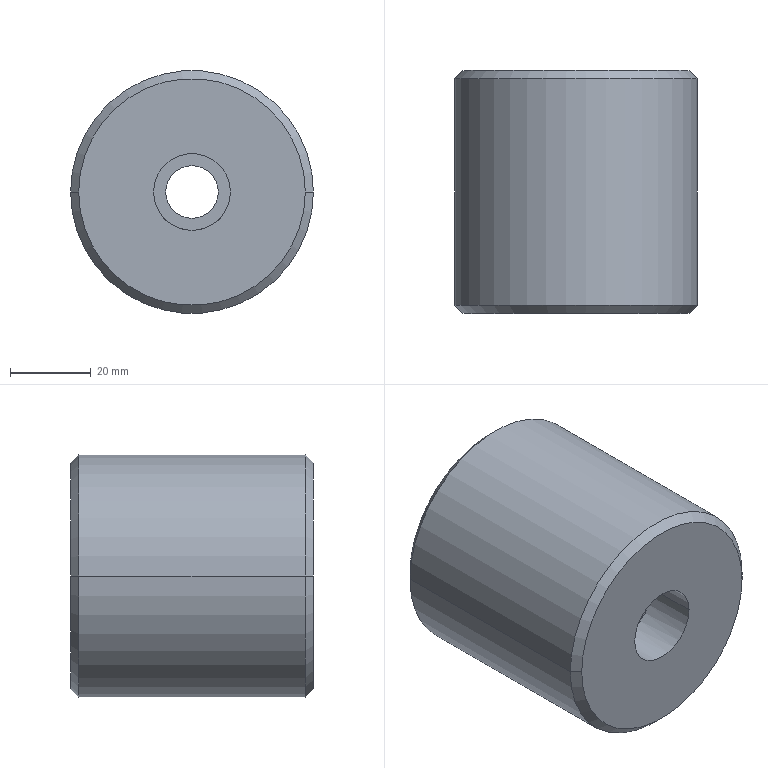Part | Creo | 1 solid | 13 faces | box 60 x 60 x 60 mm | volume 158984 mm3 | cylinder 6 | cone 4 | plane 3 | commonest cylinder face diameters 13 x2 19 x2 60 x2
STEP:
#1=CARTESIAN_POINT('',(278.,-435.005,80.));
#2=VERTEX_POINT('',#1);
#3=CARTESIAN_POINT('',(222.,-435.005,80.));
#4=VERTEX_POINT('',#3);
#5=CARTESIAN_POINT('',(250.,-435.005,80.));
#6=DIRECTION('',(0.,-1.,0.));
#7=DIRECTION('',(1.,0.,0.));
#8=AXIS2_PLACEMENT_3D('',#5,#6,#7);
#9=CIRCLE('',#8,28.);
#10=EDGE_CURVE('',#2,#4,#9,.T.);
#11=ORIENTED_EDGE('',*,*,#10,.F.);
#12=CARTESIAN_POINT('',(250.,-435.005,80.));
#13=DIRECTION('',(0.,-1.,0.));
#14=DIRECTION('',(-1.,0.,0.));
#15=AXIS2_PLACEMENT_3D('',#12,#13,#14);
#16=CIRCLE('',#15,28.);
#17=EDGE_CURVE('',#4,#2,#16,.T.);
#18=ORIENTED_EDGE('',*,*,#17,.F.);
#19=EDGE_LOOP('',(#11,#18));
#20=FACE_OUTER_BOUND('',#19,.F.);
#21=CARTESIAN_POINT('',(250.,-435.005,70.5));
#22=VERTEX_POINT('',#21);
#23=CARTESIAN_POINT('',(240.5,-435.005,80.));
#24=VERTEX_POINT('',#23);
#25=CARTESIAN_POINT('',(250.,-435.005,80.));
#26=DIRECTION('',(0.,1.,0.));
#27=DIRECTION('',(0.,0.,-1.));
#28=AXIS2_PLACEMENT_3D('',#25,#26,#27);
#29=CIRCLE('',#28,9.5);
#30=EDGE_CURVE('',#22,#24,#29,.T.);
#31=ORIENTED_EDGE('',*,*,#30,.F.);
#32=CARTESIAN_POINT('',(259.5,-435.005,80.));
#33=VERTEX_POINT('',#32);
#34=CARTESIAN_POINT('',(250.,-435.005,80.));
#35=DIRECTION('',(0.,1.,0.));
#36=DIRECTION('',(1.,0.,0.));
#37=AXIS2_PLACEMENT_3D('',#34,#35,#36);
#38=CIRCLE('',#37,9.5);
#39=EDGE_CURVE('',#33,#22,#38,.T.);
#40=ORIENTED_EDGE('',*,*,#39,.F.);
#41=CARTESIAN_POINT('',(250.,-435.005,80.));
#42=DIRECTION('',(0.,1.,0.));
#43=DIRECTION('',(-1.,0.,0.));
#44=AXIS2_PLACEMENT_3D('',#41,#42,#43);
#45=CIRCLE('',#44,9.5);
#46=EDGE_CURVE('',#24,#33,#45,.T.);
#47=ORIENTED_EDGE('',*,*,#46,.F.);
#48=EDGE_LOOP('',(#31,#40,#47));
#49=FACE_BOUND('',#48,.F.);
#50=CARTESIAN_POINT('',(10.,-435.005,-351.));
#51=DIRECTION('',(0.,-1.,0.));
#52=DIRECTION('',(1.,0.,0.));
#53=AXIS2_PLACEMENT_3D('',#50,#51,#52);
#54=PLANE('',#53);
#55=ADVANCED_FACE('',(#20,#49),#54,.T.);
#56=ORIENTED_EDGE('',*,*,#39,.T.);
#57=ORIENTED_EDGE('',*,*,#30,.T.);
#58=CARTESIAN_POINT('',(240.5,-422.005,80.));
#59=VERTEX_POINT('',#58);
#60=CARTESIAN_POINT('',(240.5,-435.005,80.));
#61=DIRECTION('',(0.,1.,0.));
#62=VECTOR('',#61,13.);
#63=LINE('',#60,#62);
#64=EDGE_CURVE('',#24,#59,#63,.T.);
#65=ORIENTED_EDGE('',*,*,#64,.T.);
#66=CARTESIAN_POINT('',(259.5,-422.005,80.));
#67=VERTEX_POINT('',#66);
#68=CARTESIAN_POINT('',(250.,-422.005,80.));
#69=DIRECTION('',(0.,-1.,0.));
#70=DIRECTION('',(-1.,0.,0.));
#71=AXIS2_PLACEMENT_3D('',#68,#69,#70);
#72=CIRCLE('',#71,9.5);
#73=EDGE_CURVE('',#59,#67,#72,.T.);
#74=ORIENTED_EDGE('',*,*,#73,.T.);
#75=CARTESIAN_POINT('',(259.5,-435.005,80.));
#76=DIRECTION('',(0.,1.,0.));
#77=VECTOR('',#76,13.);
#78=LINE('',#75,#77);
#79=EDGE_CURVE('',#33,#67,#78,.T.);
#80=ORIENTED_EDGE('',*,*,#79,.F.);
#81=EDGE_LOOP('',(#56,#57,#65,#74,#80));
#82=FACE_OUTER_BOUND('',#81,.F.);
#83=CARTESIAN_POINT('',(250.,-447.005,80.));
#84=DIRECTION('',(0.,1.,0.));
#85=DIRECTION('',(1.,0.,0.));
#86=AXIS2_PLACEMENT_3D('',#83,#84,#85);
#87=CYLINDRICAL_SURFACE('',#86,9.5);
#88=ADVANCED_FACE('',(#82),#87,.F.);
#89=ORIENTED_EDGE('',*,*,#46,.T.);
#90=ORIENTED_EDGE('',*,*,#79,.T.);
#91=CARTESIAN_POINT('',(250.,-422.005,80.));
#92=DIRECTION('',(0.,-1.,0.));
#93=DIRECTION('',(1.,0.,0.));
#94=AXIS2_PLACEMENT_3D('',#91,#92,#93);
#95=CIRCLE('',#94,9.5);
#96=EDGE_CURVE('',#67,#59,#95,.T.);
#97=ORIENTED_EDGE('',*,*,#96,.T.);
#98=ORIENTED_EDGE('',*,*,#64,.F.);
#99=EDGE_LOOP('',(#89,#90,#97,#98));
#100=FACE_OUTER_BOUND('',#99,.F.);
#101=CARTESIAN_POINT('',(250.,-447.005,80.));
#102=DIRECTION('',(0.,1.,0.));
#103=DIRECTION('',(1.,0.,0.));
#104=AXIS2_PLACEMENT_3D('',#101,#102,#103);
#105=CYLINDRICAL_SURFACE('',#104,9.5);
#106=ADVANCED_FACE('',(#100),#105,.F.);
#107=ORIENTED_EDGE('',*,*,#96,.F.);
#108=ORIENTED_EDGE('',*,*,#73,.F.);
#109=EDGE_LOOP('',(#107,#108));
#110=FACE_OUTER_BOUND('',#109,.F.);
#111=CARTESIAN_POINT('',(250.,-422.005,86.5));
#112=VERTEX_POINT('',#111);
#113=CARTESIAN_POINT('',(256.5,-422.005,80.));
#114=VERTEX_POINT('',#113);
#115=CARTESIAN_POINT('',(250.,-422.005,80.));
#116=DIRECTION('',(0.,1.,0.));
#117=DIRECTION('',(0.,0.,1.));
#118=AXIS2_PLACEMENT_3D('',#115,#116,#117);
#119=CIRCLE('',#118,6.5);
#120=EDGE_CURVE('',#112,#114,#119,.T.);
#121=ORIENTED_EDGE('',*,*,#120,.F.);
#122=CARTESIAN_POINT('',(243.5,-422.005,80.));
#123=VERTEX_POINT('',#122);
#124=CARTESIAN_POINT('',(250.,-422.005,80.));
#125=DIRECTION('',(0.,1.,0.));
#126=DIRECTION('',(-1.,0.,0.));
#127=AXIS2_PLACEMENT_3D('',#124,#125,#126);
#128=CIRCLE('',#127,6.5);
#129=EDGE_CURVE('',#123,#112,#128,.T.);
#130=ORIENTED_EDGE('',*,*,#129,.F.);
#131=CARTESIAN_POINT('',(250.,-422.005,73.5));
#132=VERTEX_POINT('',#131);
#133=CARTESIAN_POINT('',(250.,-422.005,80.));
#134=DIRECTION('',(0.,1.,0.));
#135=DIRECTION('',(0.,0.,-1.));
#136=AXIS2_PLACEMENT_3D('',#133,#134,#135);
#137=CIRCLE('',#136,6.5);
#138=EDGE_CURVE('',#132,#123,#137,.T.);
#139=ORIENTED_EDGE('',*,*,#138,.F.);
#140=CARTESIAN_POINT('',(250.,-422.005,80.));
#141=DIRECTION('',(0.,1.,0.));
#142=DIRECTION('',(1.,0.,0.));
#143=AXIS2_PLACEMENT_3D('',#140,#141,#142);
#144=CIRCLE('',#143,6.5);
#145=EDGE_CURVE('',#114,#132,#144,.T.);
#146=ORIENTED_EDGE('',*,*,#145,.F.);
#147=EDGE_LOOP('',(#121,#130,#139,#146));
#148=FACE_BOUND('',#147,.F.);
#149=CARTESIAN_POINT('',(250.,-422.005,80.));
#150=DIRECTION('',(0.,1.,0.));
#151=DIRECTION('',(0.,0.,1.));
#152=AXIS2_PLACEMENT_3D('',#149,#150,#151);
#153=PLANE('',#152);
#154=ADVANCED_FACE('',(#110,#148),#153,.F.);
#155=ORIENTED_EDGE('',*,*,#129,.T.);
#156=ORIENTED_EDGE('',*,*,#120,.T.);
#157=CARTESIAN_POINT('',(256.5,-375.005,80.));
#158=VERTEX_POINT('',#157);
#159=CARTESIAN_POINT('',(256.5,-422.005,80.));
#160=DIRECTION('',(0.,1.,0.));
#161=VECTOR('',#160,47.);
#162=LINE('',#159,#161);
#163=EDGE_CURVE('',#114,#158,#162,.T.);
#164=ORIENTED_EDGE('',*,*,#163,.T.);
#165=CARTESIAN_POINT('',(243.5,-375.005,80.));
#166=VERTEX_POINT('',#165);
#167=CARTESIAN_POINT('',(250.,-375.005,80.));
#168=DIRECTION('',(0.,-1.,0.));
#169=DIRECTION('',(1.,0.,0.));
#170=AXIS2_PLACEMENT_3D('',#167,#168,#169);
#171=CIRCLE('',#170,6.5);
#172=EDGE_CURVE('',#158,#166,#171,.T.);
#173=ORIENTED_EDGE('',*,*,#172,.T.);
#174=CARTESIAN_POINT('',(243.5,-422.005,80.));
#175=DIRECTION('',(0.,1.,0.));
#176=VECTOR('',#175,47.);
#177=LINE('',#174,#176);
#178=EDGE_CURVE('',#123,#166,#177,.T.);
#179=ORIENTED_EDGE('',*,*,#178,.F.);
#180=EDGE_LOOP('',(#155,#156,#164,#173,#179));
#181=FACE_OUTER_BOUND('',#180,.F.);
#182=CARTESIAN_POINT('',(250.,-447.005,80.));
#183=DIRECTION('',(0.,1.,0.));
#184=DIRECTION('',(1.,0.,0.));
#185=AXIS2_PLACEMENT_3D('',#182,#183,#184);
#186=CYLINDRICAL_SURFACE('',#185,6.5);
#187=ADVANCED_FACE('',(#181),#186,.F.);
#188=ORIENTED_EDGE('',*,*,#138,.T.);
#189=ORIENTED_EDGE('',*,*,#178,.T.);
#190=CARTESIAN_POINT('',(250.,-375.005,80.));
#191=DIRECTION('',(0.,-1.,0.));
#192=DIRECTION('',(-1.,0.,0.));
#193=AXIS2_PLACEMENT_3D('',#190,#191,#192);
#194=CIRCLE('',#193,6.5);
#195=EDGE_CURVE('',#166,#158,#194,.T.);
#196=ORIENTED_EDGE('',*,*,#195,.T.);
#197=ORIENTED_EDGE('',*,*,#163,.F.);
#198=ORIENTED_EDGE('',*,*,#145,.T.);
#199=EDGE_LOOP('',(#188,#189,#196,#197,#198));
#200=FACE_OUTER_BOUND('',#199,.F.);
#201=CARTESIAN_POINT('',(250.,-447.005,80.));
#202=DIRECTION('',(0.,1.,0.));
#203=DIRECTION('',(1.,0.,0.));
#204=AXIS2_PLACEMENT_3D('',#201,#202,#203);
#205=CYLINDRICAL_SURFACE('',#204,6.5);
#206=ADVANCED_FACE('',(#200),#205,.F.);
#207=CARTESIAN_POINT('',(222.,-375.005,80.));
#208=VERTEX_POINT('',#207);
#209=CARTESIAN_POINT('',(278.,-375.005,80.));
#210=VERTEX_POINT('',#209);
#211=CARTESIAN_POINT('',(250.,-375.005,80.));
#212=DIRECTION('',(0.,1.,0.));
#213=DIRECTION('',(-1.,0.,0.));
#214=AXIS2_PLACEMENT_3D('',#211,#212,#213);
#215=CIRCLE('',#214,28.);
#216=EDGE_CURVE('',#208,#210,#215,.T.);
#217=ORIENTED_EDGE('',*,*,#216,.F.);
#218=CARTESIAN_POINT('',(250.,-375.005,80.));
#219=DIRECTION('',(0.,1.,0.));
#220=DIRECTION('',(1.,0.,0.));
#221=AXIS2_PLACEMENT_3D('',#218,#219,#220);
#222=CIRCLE('',#221,28.);
#223=EDGE_CURVE('',#210,#208,#222,.T.);
#224=ORIENTED_EDGE('',*,*,#223,.F.);
#225=EDGE_LOOP('',(#217,#224));
#226=FACE_OUTER_BOUND('',#225,.F.);
#227=ORIENTED_EDGE('',*,*,#172,.F.);
#228=ORIENTED_EDGE('',*,*,#195,.F.);
#229=EDGE_LOOP('',(#227,#228));
#230=FACE_BOUND('',#229,.F.);
#231=CARTESIAN_POINT('',(10.,-375.005,-351.));
#232=DIRECTION('',(0.,-1.,0.));
#233=DIRECTION('',(1.,0.,0.));
#234=AXIS2_PLACEMENT_3D('',#231,#232,#233);
#235=PLANE('',#234);
#236=ADVANCED_FACE('',(#226,#230),#235,.F.);
#237=CARTESIAN_POINT('',(220.,-377.005,80.));
#238=VERTEX_POINT('',#237);
#239=CARTESIAN_POINT('',(280.,-377.005,80.));
#240=VERTEX_POINT('',#239);
#241=CARTESIAN_POINT('',(250.,-377.005,80.));
#242=DIRECTION('',(0.,1.,0.));
#243=DIRECTION('',(-1.,0.,0.));
#244=AXIS2_PLACEMENT_3D('',#241,#242,#243);
#245=CIRCLE('',#244,30.);
#246=EDGE_CURVE('',#238,#240,#245,.T.);
#247=ORIENTED_EDGE('',*,*,#246,.F.);
#248=CARTESIAN_POINT('',(222.,-375.005,80.));
#249=DIRECTION('',(-0.7071,-0.7071,0.));
#250=VECTOR('',#249,2.828);
#251=LINE('',#248,#250);
#252=EDGE_CURVE('',#208,#238,#251,.T.);
#253=ORIENTED_EDGE('',*,*,#252,.F.);
#254=ORIENTED_EDGE('',*,*,#216,.T.);
#255=CARTESIAN_POINT('',(278.,-375.005,80.));
#256=DIRECTION('',(0.7071,-0.7071,0.));
#257=VECTOR('',#256,2.828);
#258=LINE('',#255,#257);
#259=EDGE_CURVE('',#210,#240,#258,.T.);
#260=ORIENTED_EDGE('',*,*,#259,.T.);
#261=EDGE_LOOP('',(#247,#253,#254,#260));
#262=FACE_OUTER_BOUND('',#261,.F.);
#263=CARTESIAN_POINT('',(250.,-376.005,80.));
#264=DIRECTION('',(0.,-1.,0.));
#265=DIRECTION('',(-1.,0.,0.));
#266=AXIS2_PLACEMENT_3D('',#263,#264,#265);
#267=CONICAL_SURFACE('',#266,29.,45.);
#268=ADVANCED_FACE('',(#262),#267,.T.);
#269=ORIENTED_EDGE('',*,*,#246,.T.);
#270=CARTESIAN_POINT('',(280.,-433.005,80.));
#271=VERTEX_POINT('',#270);
#272=CARTESIAN_POINT('',(280.,-377.005,80.));
#273=DIRECTION('',(0.,-1.,0.));
#274=VECTOR('',#273,56.);
#275=LINE('',#272,#274);
#276=EDGE_CURVE('',#240,#271,#275,.T.);
#277=ORIENTED_EDGE('',*,*,#276,.T.);
#278=CARTESIAN_POINT('',(220.,-433.005,80.));
#279=VERTEX_POINT('',#278);
#280=CARTESIAN_POINT('',(250.,-433.005,80.));
#281=DIRECTION('',(0.,-1.,0.));
#282=DIRECTION('',(1.,0.,0.));
#283=AXIS2_PLACEMENT_3D('',#280,#281,#282);
#284=CIRCLE('',#283,30.);
#285=EDGE_CURVE('',#271,#279,#284,.T.);
#286=ORIENTED_EDGE('',*,*,#285,.T.);
#287=CARTESIAN_POINT('',(220.,-377.005,80.));
#288=DIRECTION('',(0.,-1.,0.));
#289=VECTOR('',#288,56.);
#290=LINE('',#287,#289);
#291=EDGE_CURVE('',#238,#279,#290,.T.);
#292=ORIENTED_EDGE('',*,*,#291,.F.);
#293=EDGE_LOOP('',(#269,#277,#286,#292));
#294=FACE_OUTER_BOUND('',#293,.F.);
#295=CARTESIAN_POINT('',(250.,-375.005,80.));
#296=DIRECTION('',(0.,-1.,0.));
#297=DIRECTION('',(1.,0.,0.));
#298=AXIS2_PLACEMENT_3D('',#295,#296,#297);
#299=CYLINDRICAL_SURFACE('',#298,30.);
#300=ADVANCED_FACE('',(#294),#299,.T.);
#301=CARTESIAN_POINT('',(250.,-377.005,80.));
#302=DIRECTION('',(0.,1.,0.));
#303=DIRECTION('',(1.,0.,0.));
#304=AXIS2_PLACEMENT_3D('',#301,#302,#303);
#305=CIRCLE('',#304,30.);
#306=EDGE_CURVE('',#240,#238,#305,.T.);
#307=ORIENTED_EDGE('',*,*,#306,.T.);
#308=ORIENTED_EDGE('',*,*,#291,.T.);
#309=CARTESIAN_POINT('',(250.,-433.005,80.));
#310=DIRECTION('',(0.,-1.,0.));
#311=DIRECTION('',(-1.,0.,0.));
#312=AXIS2_PLACEMENT_3D('',#309,#310,#311);
#313=CIRCLE('',#312,30.);
#314=EDGE_CURVE('',#279,#271,#313,.T.);
#315=ORIENTED_EDGE('',*,*,#314,.T.);
#316=ORIENTED_EDGE('',*,*,#276,.F.);
#317=EDGE_LOOP('',(#307,#308,#315,#316));
#318=FACE_OUTER_BOUND('',#317,.F.);
#319=CARTESIAN_POINT('',(250.,-375.005,80.));
#320=DIRECTION('',(0.,-1.,0.));
#321=DIRECTION('',(1.,0.,0.));
#322=AXIS2_PLACEMENT_3D('',#319,#320,#321);
#323=CYLINDRICAL_SURFACE('',#322,30.);
#324=ADVANCED_FACE('',(#318),#323,.T.);
#325=ORIENTED_EDGE('',*,*,#306,.F.);
#326=ORIENTED_EDGE('',*,*,#259,.F.);
#327=ORIENTED_EDGE('',*,*,#223,.T.);
#328=ORIENTED_EDGE('',*,*,#252,.T.);
#329=EDGE_LOOP('',(#325,#326,#327,#328));
#330=FACE_OUTER_BOUND('',#329,.F.);
#331=CARTESIAN_POINT('',(250.,-376.005,80.));
#332=DIRECTION('',(0.,-1.,0.));
#333=DIRECTION('',(-1.,0.,0.));
#334=AXIS2_PLACEMENT_3D('',#331,#332,#333);
#335=CONICAL_SURFACE('',#334,29.,45.);
#336=ADVANCED_FACE('',(#330),#335,.T.);
#337=ORIENTED_EDGE('',*,*,#17,.T.);
#338=CARTESIAN_POINT('',(278.,-435.005,80.));
#339=DIRECTION('',(0.7071,0.7071,0.));
#340=VECTOR('',#339,2.828);
#341=LINE('',#338,#340);
#342=EDGE_CURVE('',#2,#271,#341,.T.);
#343=ORIENTED_EDGE('',*,*,#342,.T.);
#344=ORIENTED_EDGE('',*,*,#314,.F.);
#345=CARTESIAN_POINT('',(222.,-435.005,80.));
#346=DIRECTION('',(-0.7071,0.7071,0.));
#347=VECTOR('',#346,2.828);
#348=LINE('',#345,#347);
#349=EDGE_CURVE('',#4,#279,#348,.T.);
#350=ORIENTED_EDGE('',*,*,#349,.F.);
#351=EDGE_LOOP('',(#337,#343,#344,#350));
#352=FACE_OUTER_BOUND('',#351,.F.);
#353=CARTESIAN_POINT('',(250.,-434.005,80.));
#354=DIRECTION('',(0.,1.,0.));
#355=DIRECTION('',(-1.,0.,0.));
#356=AXIS2_PLACEMENT_3D('',#353,#354,#355);
#357=CONICAL_SURFACE('',#356,29.,45.);
#358=ADVANCED_FACE('',(#352),#357,.T.);
#359=ORIENTED_EDGE('',*,*,#10,.T.);
#360=ORIENTED_EDGE('',*,*,#349,.T.);
#361=ORIENTED_EDGE('',*,*,#285,.F.);
#362=ORIENTED_EDGE('',*,*,#342,.F.);
#363=EDGE_LOOP('',(#359,#360,#361,#362));
#364=FACE_OUTER_BOUND('',#363,.F.);
#365=CARTESIAN_POINT('',(250.,-434.005,80.));
#366=DIRECTION('',(0.,1.,0.));
#367=DIRECTION('',(-1.,0.,0.));
#368=AXIS2_PLACEMENT_3D('',#365,#366,#367);
#369=CONICAL_SURFACE('',#368,29.,45.);
#370=ADVANCED_FACE('',(#364),#369,.T.);
#371=CLOSED_SHELL('',(#55,#88,#106,#154,#187,#206,#236,#268,#300,#324,#336,#358,#370));
#372=MANIFOLD_SOLID_BREP('',#371);
#373=(LENGTH_UNIT()NAMED_UNIT(*)SI_UNIT(.MILLI.,.METRE.));
#374=UNCERTAINTY_MEASURE_WITH_UNIT(LENGTH_MEASURE(0.01039),#373,'','');
#375=(NAMED_UNIT(*)PLANE_ANGLE_UNIT()SI_UNIT($,.RADIAN.));
#376=PLANE_ANGLE_MEASURE_WITH_UNIT(PLANE_ANGLE_MEASURE(0.01745),#375);
#377=(CONVERSION_BASED_UNIT('DEGREE',#376)NAMED_UNIT(*)PLANE_ANGLE_UNIT());
#378=(NAMED_UNIT(*)SI_UNIT($,.STERADIAN.)SOLID_ANGLE_UNIT());
#379=(GEOMETRIC_REPRESENTATION_CONTEXT(3)GLOBAL_UNCERTAINTY_ASSIGNED_CONTEXT((#374))GLOBAL_UNIT_ASSIGNED_CONTEXT((#373,#377,#378))REPRESENTATION_CONTEXT('',''));
#380=ADVANCED_BREP_SHAPE_REPRESENTATION('',(#372),#379);